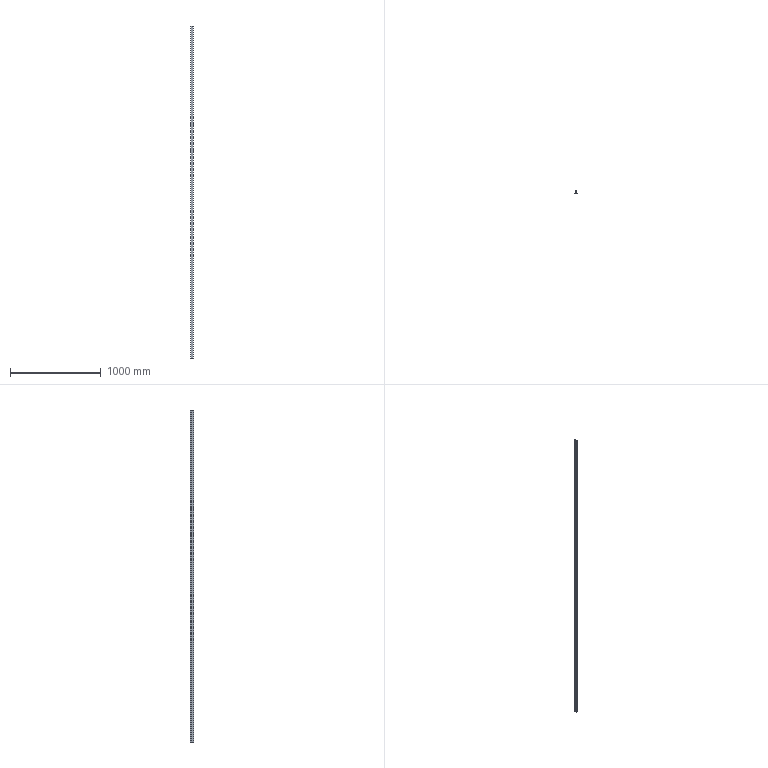Part | STEP file | Thanh T chinh 3m6 | 1 solid | 20 faces | box 24 x 37.5 x 3660 mm | volume 442294 mm3 | plane 14 | cylinder 6 | commonest cylinder face diameters 1.2 x6